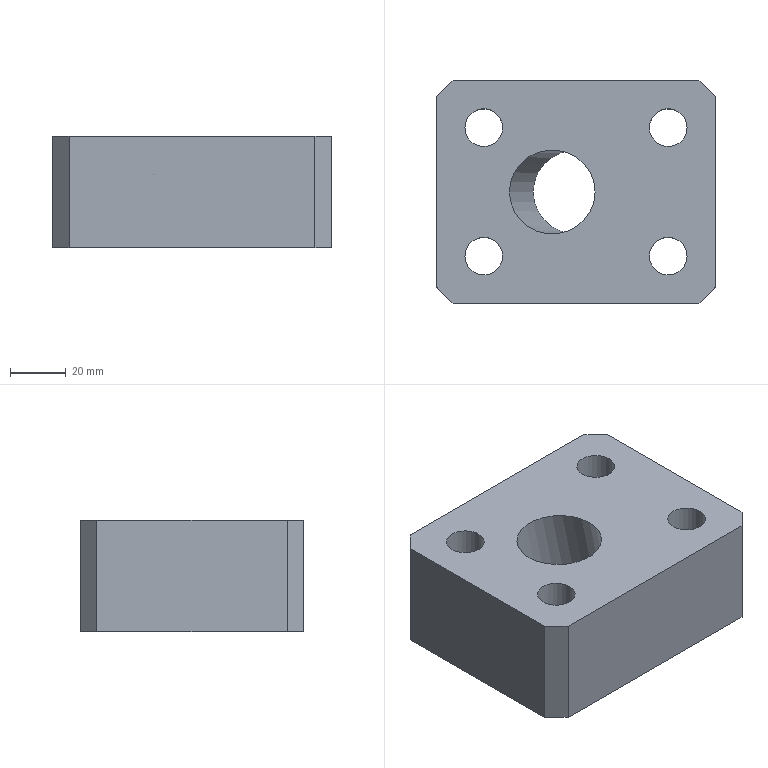Part | STEP file | solid 81 | 1 solid | 23 faces | box 100 x 80 x 40 mm | volume 256419 mm3 | plane 14 | cylinder 9 | commonest cylinder face diameters 13.5 x4 20 x4 30 x1